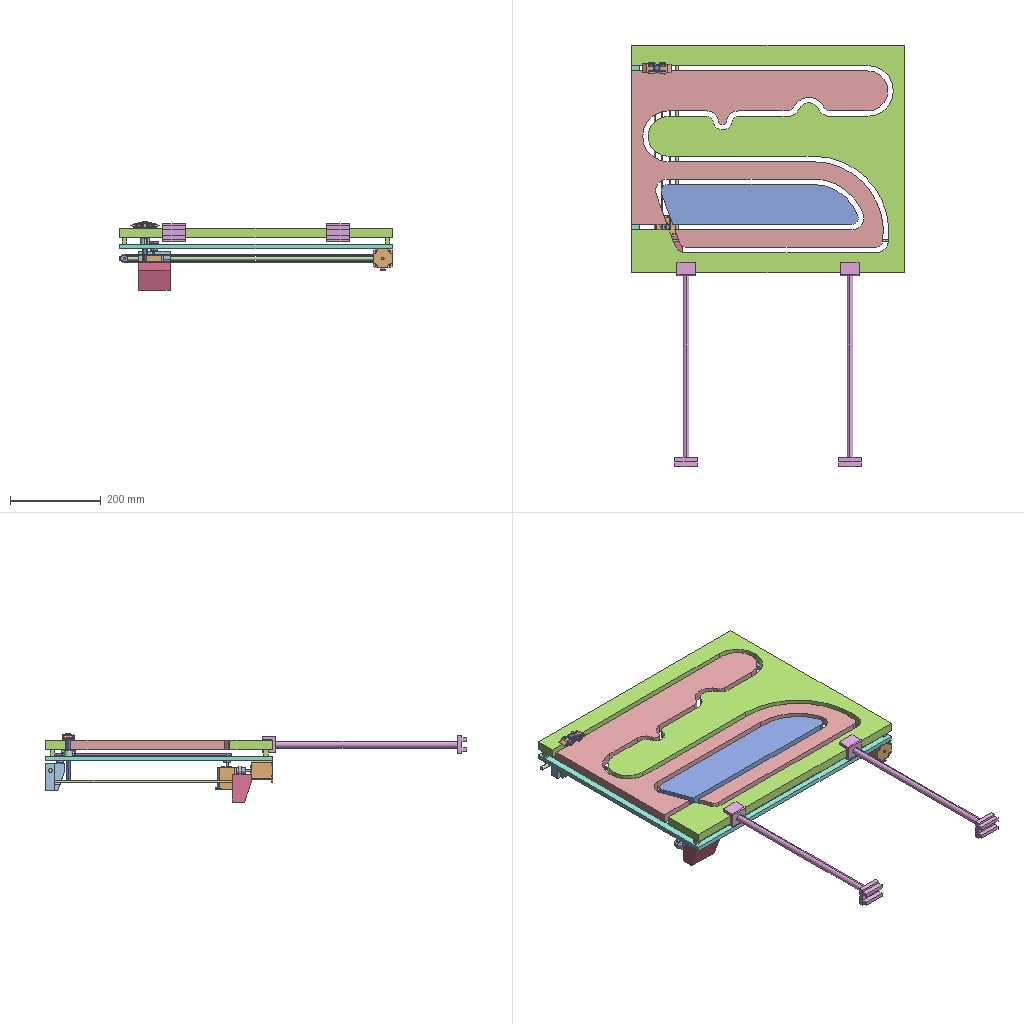Assembly | SolidWorks | 16 different items | 22 placed | box 600 x 927 x 150 mm
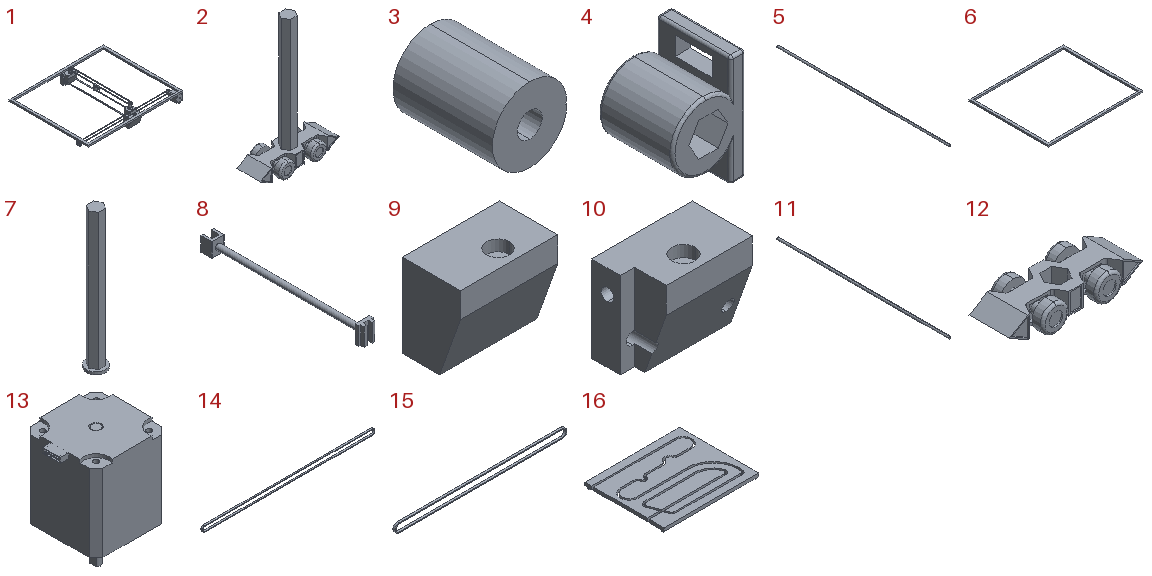Parts list (item | name | quantity | parent item | size | volume | features):
1 | (subassembly) | x1 | - | 600 x 500 x 111.5 mm | 820958 mm3 | -
2 | (subassembly) | x1 | - | 62.5 x 25 x 103 mm | 16167 mm3 | features CompositeCurve 4
3 | - | x4 | in 1 | 15 x 20 x 15 mm | 3140 mm3 | features Extrusion 1, ICE 1
4 | - | x1 | in 1 | 19.787 x 20 x 30 mm | 5242 mm3 | features ICE 3, Fillet 2, Extrusion 1, MirrorPattern 1
5 | - | x2 | in 1 | 5 x 420 x 5 mm | 8247 mm3 | features Extrusion 1
6 | - | x1 | in 1 | 600 x 500 x 10 mm | 317236 mm3 | features Extrusion 1
7 | - | x1 | in 2 | 14 x 14 x 103 mm | 7725 mm3 | features Chamfer 1, Extrusion 1, ICE 1
8 | - | x2 | - | 40 x 450 x 50 mm | 121566 mm3 | features ICE 3, Extrusion 1, Fillet 1
9 | - | x1 | in 1 | 70 x 42 x 60 mm | 152639 mm3 | features ICE 2, Extrusion 1
10 | - | x1 | in 1 | 70 x 42 x 60 mm | 135372 mm3 | features ICE 4, Extrusion 1
11 | - | x1 | - | 8 x 600 x 8 mm | 30159 mm3 | features Extrusion 1
12 | - | x1 | in 2 | 62.5 x 25 x 12.5 mm | 8442 mm3 | features ICE 8, MirrorPattern 3, Chamfer 1, Extrusion 1, Fillet 1, Scale 1
13 | - | x2 | in 1 | 47 x 42 x 69 mm | 80717 mm3 | features ICE 8, Extrusion 1
14 | - | x1 | in 1 | 588 x 5 x 19 mm | 11914 mm3 | features Extrusion 1
15 | - | x1 | in 1 | 395 x 5 x 20 mm | 8065 mm3 | features Extrusion 1
16 | - | x1 | - | 600 x 500 x 35 mm | 5161469 mm3 | features ICE 4, CutThin 2, MirrorPattern 2, Extrusion 1
Mates (type | each side: item.copy, entity, surface, feature):
In the top assembly
Coincident | 16.1 face plane Boss-Extrude1 | 8.1 face plane Boss-Extrude1 | 2 times
Coincident | 16.1 face plane Boss-Extrude1 | 8.2 face plane Boss-Extrude1 | 2 times
Symmetric | 8.1 plane | 8.2 plane | assembly plane
Coincident | 16.1 face plane Boss-Extrude1 | 6.1 face plane Boss-Extrude1 | 2 times
DistanceDim | 6.1 face plane Boss-Extrude1 | 16.1 face plane Boss-Extrude1
Coincident | 4.1 face plane Cut-Extrude1 | 7.1 face plane Boss-Extrude1 | 2 times
Tangent | 16.1 face plane Boss-Extrude1 | 12.1 face cylinder Mirror3
Concentric | 10.1 face cylinder Cut-Extrude3 | 11.1 face cylinder Boss-Extrude1
Coincident | 6.1 face plane Boss-Extrude1 | 11.1 face plane Boss-Extrude1
In subassembly 1
Coincident | 6.2 face plane Boss-Extrude1 | 13.1 face plane Boss-Extrude1 | 3 times
Concentric | 3.1 face cylinder Boss-Extrude1 | 14.1 face cylinder Boss-Extrude1
Parallel | 6.2 face plane Boss-Extrude1 | 14.1 face plane Boss-Extrude1
DistanceDim | 10.2 face plane Boss-Extrude1 | 6.2 face plane Boss-Extrude1
Coincident | 6.2 face plane Boss-Extrude1 | 10.2 face plane Boss-Extrude1
Coincident | 5.1 face plane Boss-Extrude1 | 5.2 face plane Boss-Extrude1
Concentric | 13.2 face cylinder Boss-Extrude3 | 3.2 face cylinder Boss-Extrude1
Concentric | 13.1 face cylinder Boss-Extrude3 | 3.3 face cylinder Boss-Extrude1
DistanceDim | 3.3 face plane Boss-Extrude1 | 13.1 face plane Boss-Extrude2
Coincident | 3.1 face plane Boss-Extrude1 | 3.3 face plane Boss-Extrude1
DistanceDim | 14.1 face plane Boss-Extrude1 | 3.3 face plane Boss-Extrude1
Tangent | 14.1 face plane Boss-Extrude1 | 3.3 face cylinder Boss-Extrude1
DistanceDim | 3.2 face plane Boss-Extrude1 | 13.2 face plane Boss-Extrude2
Coincident | 3.2 face plane Boss-Extrude1 | 3.4 face plane Boss-Extrude1
Coincident | 3.2 face plane Boss-Extrude1 | 15.1 face plane Boss-Extrude1
Concentric | 3.2 face cylinder Boss-Extrude1 | 15.1 face cylinder Boss-Extrude1
Tangent | 3.4 face cylinder Boss-Extrude1 | 15.1 face plane Boss-Extrude1
Coincident | 15.1 face plane Boss-Extrude1 | 4.2 face plane Boss-Extrude1
Width | 4.2 face plane Boss-Extrude1 | 4.2 face plane Boss-Extrude1 | 15.1 face plane Boss-Extrude1 | 15.1 face plane Boss-Extrude1
Concentric | 1.1 face | 3.1 face cylinder Boss-Extrude1
In subassembly 2
Concentric | 12.2 select_type:24 | 7.2 edge
Coincident | 12.2 face plane Boss-Extrude1 | 7.2 face plane Boss-Extrude2